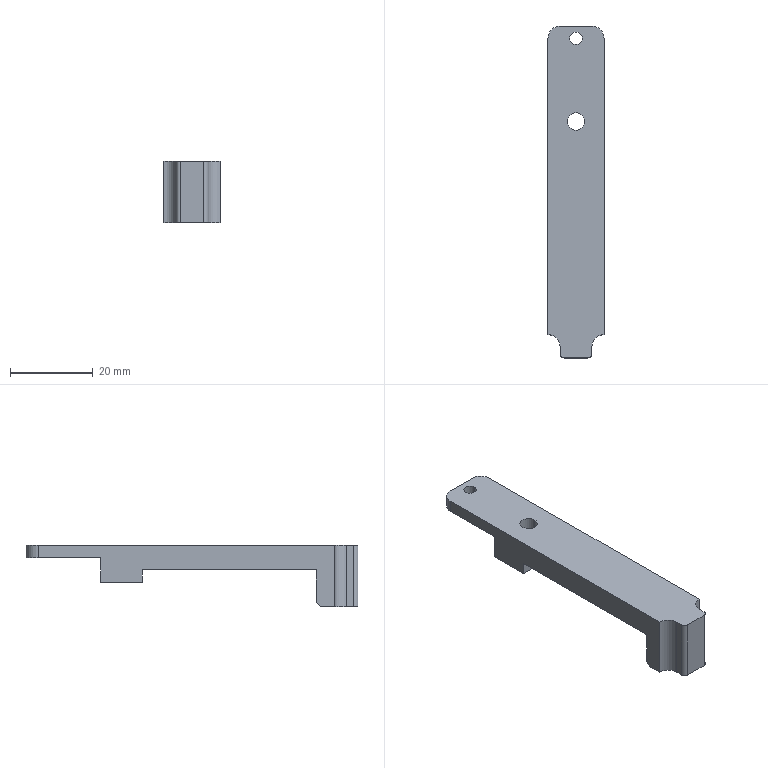Part | STEP file | QA-AD07 | 1 solid | 25 faces | box 13.5 x 80 x 14.8 mm | volume 6677 mm3 | plane 15 | cylinder 10 | commonest cylinder face diameters 2 x2 3 x2 4.2 x2 5.8 x2 6 x2